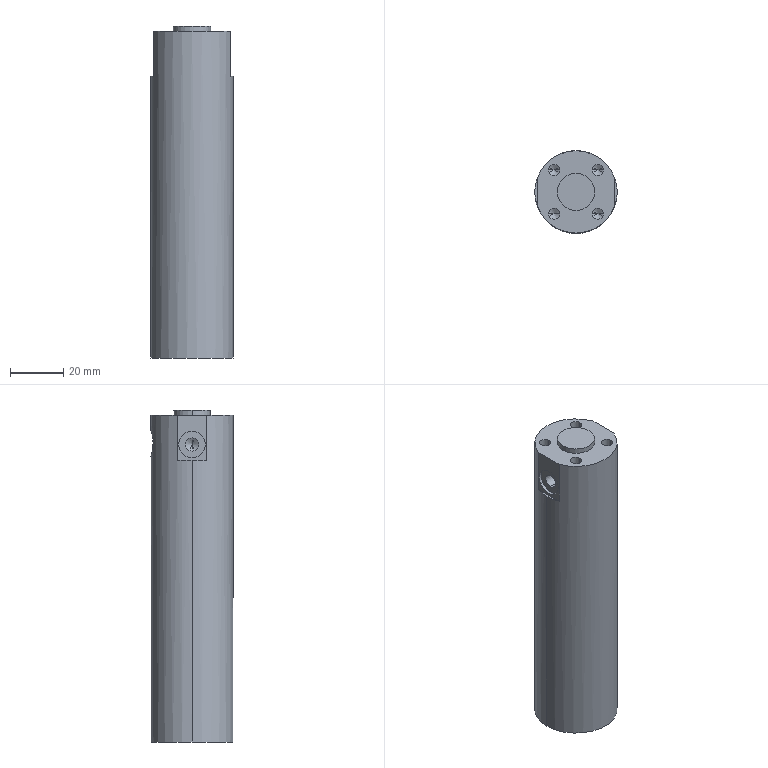Part | STEP file | 0229_Z_Cylinder_CG1DN25-75_1 | 1 solid | 54 faces | box 31 x 31 x 125 mm | volume 50538 mm3 | cylinder 28 | cone 14 | plane 12 | commonest cylinder face diameters 4.2 x8 10 x8 5 x4 6.8 x2 14 x2 25 x2